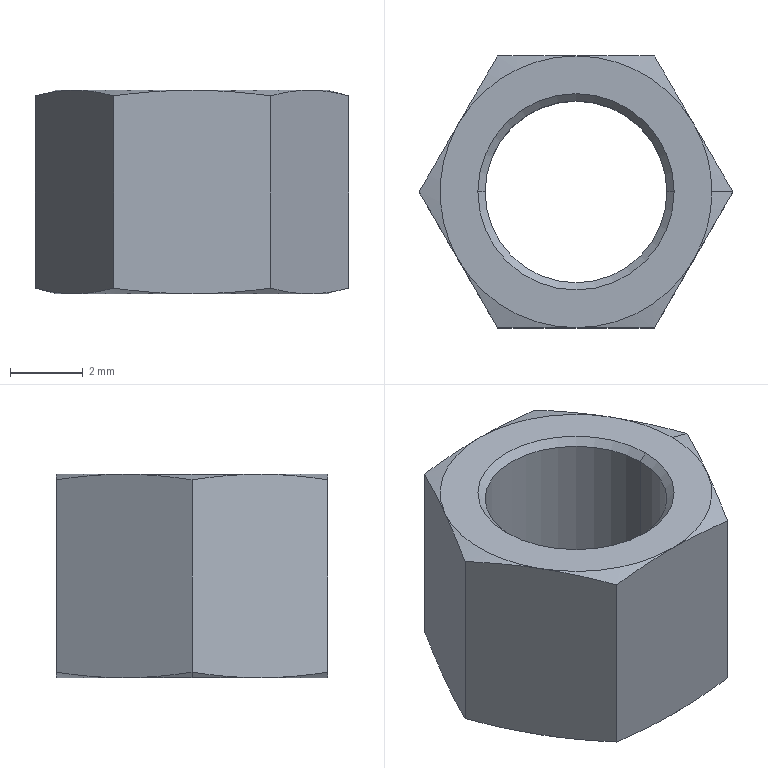Part | SolidWorks | features Cut 2, Chamfer 1, Extrusion 1 | 1 solid | 28 faces | box 8.63 x 7.474 x 5.6 mm | volume 159.862 mm3 | cone 18 | plane 8 | cylinder 2 | commonest cylinder face diameters 5 x2
STEP:
#1=CARTESIAN_POINT('',(-2.5,0.,5.4));
#2=VERTEX_POINT('',#1);
#3=CARTESIAN_POINT('',(2.5,0.,5.4));
#4=VERTEX_POINT('',#3);
#5=CARTESIAN_POINT('',(0.,0.,5.4));
#6=DIRECTION('',(0.,0.,1.));
#7=DIRECTION('',(1.,0.,0.));
#8=AXIS2_PLACEMENT_3D('',#5,#6,#7);
#9=CIRCLE('',#8,2.5);
#10=EDGE_CURVE('',#2,#4,#9,.T.);
#11=ORIENTED_EDGE('',*,*,#10,.F.);
#12=CARTESIAN_POINT('',(-2.7,0.,5.6));
#13=VERTEX_POINT('',#12);
#14=CARTESIAN_POINT('',(-2.5,0.,5.4));
#15=DIRECTION('',(-0.7071,0.,0.7071));
#16=VECTOR('',#15,1000.);
#17=LINE('',#14,#16);
#18=EDGE_CURVE('',#2,#13,#17,.T.);
#19=ORIENTED_EDGE('',*,*,#18,.T.);
#20=CARTESIAN_POINT('',(2.7,0.,5.6));
#21=VERTEX_POINT('',#20);
#22=CARTESIAN_POINT('',(0.,0.,5.6));
#23=DIRECTION('',(0.,0.,-1.));
#24=DIRECTION('',(1.,0.,0.));
#25=AXIS2_PLACEMENT_3D('',#22,#23,#24);
#26=CIRCLE('',#25,2.7);
#27=EDGE_CURVE('',#21,#13,#26,.T.);
#28=ORIENTED_EDGE('',*,*,#27,.F.);
#29=CARTESIAN_POINT('',(2.5,0.,5.4));
#30=DIRECTION('',(0.7071,0.,0.7071));
#31=VECTOR('',#30,1000.);
#32=LINE('',#29,#31);
#33=EDGE_CURVE('',#4,#21,#32,.T.);
#34=ORIENTED_EDGE('',*,*,#33,.F.);
#35=EDGE_LOOP('',(#11,#19,#28,#34));
#36=FACE_OUTER_BOUND('',#35,.T.);
#37=CARTESIAN_POINT('',(0.,0.,5.4));
#38=DIRECTION('',(0.,0.,1.));
#39=DIRECTION('',(1.,0.,0.));
#40=AXIS2_PLACEMENT_3D('',#37,#38,#39);
#41=CONICAL_SURFACE('',#40,2.5,0.7854);
#42=ADVANCED_FACE('',(#36),#41,.F.);
#43=CARTESIAN_POINT('',(2.5,0.,0.2));
#44=VERTEX_POINT('',#43);
#45=CARTESIAN_POINT('',(-2.5,0.,0.2));
#46=VERTEX_POINT('',#45);
#47=CARTESIAN_POINT('',(0.,0.,0.2));
#48=DIRECTION('',(0.,0.,-1.));
#49=DIRECTION('',(1.,0.,0.));
#50=AXIS2_PLACEMENT_3D('',#47,#48,#49);
#51=CIRCLE('',#50,2.5);
#52=EDGE_CURVE('',#44,#46,#51,.T.);
#53=ORIENTED_EDGE('',*,*,#52,.F.);
#54=CARTESIAN_POINT('',(2.7,0.,0.));
#55=VERTEX_POINT('',#54);
#56=CARTESIAN_POINT('',(2.7,0.,0.));
#57=DIRECTION('',(0.7071,0.,-0.7071));
#58=VECTOR('',#57,1000.);
#59=LINE('',#56,#58);
#60=EDGE_CURVE('',#44,#55,#59,.T.);
#61=ORIENTED_EDGE('',*,*,#60,.T.);
#62=CARTESIAN_POINT('',(-2.7,0.,0.));
#63=VERTEX_POINT('',#62);
#64=CARTESIAN_POINT('',(0.,0.,0.));
#65=DIRECTION('',(0.,0.,1.));
#66=DIRECTION('',(1.,0.,0.));
#67=AXIS2_PLACEMENT_3D('',#64,#65,#66);
#68=CIRCLE('',#67,2.7);
#69=EDGE_CURVE('',#63,#55,#68,.T.);
#70=ORIENTED_EDGE('',*,*,#69,.F.);
#71=CARTESIAN_POINT('',(-2.7,0.,0.));
#72=DIRECTION('',(-0.7071,0.,-0.7071));
#73=VECTOR('',#72,1000.);
#74=LINE('',#71,#73);
#75=EDGE_CURVE('',#46,#63,#74,.T.);
#76=ORIENTED_EDGE('',*,*,#75,.F.);
#77=EDGE_LOOP('',(#53,#61,#70,#76));
#78=FACE_OUTER_BOUND('',#77,.T.);
#79=CARTESIAN_POINT('',(0.,0.,0.));
#80=DIRECTION('',(0.,0.,-1.));
#81=DIRECTION('',(-1.,0.,0.));
#82=AXIS2_PLACEMENT_3D('',#79,#80,#81);
#83=CONICAL_SURFACE('',#82,2.7,0.7854);
#84=ADVANCED_FACE('',(#78),#83,.F.);
#85=CARTESIAN_POINT('',(3.737,0.,5.6));
#86=VERTEX_POINT('',#85);
#87=CARTESIAN_POINT('',(3.236,1.868,5.6));
#88=VERTEX_POINT('',#87);
#89=CARTESIAN_POINT('',(0.,0.,5.6));
#90=DIRECTION('',(0.,0.,1.));
#91=DIRECTION('',(1.,0.,0.));
#92=AXIS2_PLACEMENT_3D('',#89,#90,#91);
#93=CIRCLE('',#92,3.737);
#94=EDGE_CURVE('',#86,#88,#93,.T.);
#95=ORIENTED_EDGE('',*,*,#94,.F.);
#96=CARTESIAN_POINT('',(4.315,0.,5.445));
#97=VERTEX_POINT('',#96);
#98=CARTESIAN_POINT('',(3.737,0.,5.6));
#99=DIRECTION('',(0.9659,0.,-0.2588));
#100=VECTOR('',#99,1000.);
#101=LINE('',#98,#100);
#102=EDGE_CURVE('',#86,#97,#101,.T.);
#103=ORIENTED_EDGE('',*,*,#102,.T.);
#104=CARTESIAN_POINT('',(4.315,0.,5.445));
#105=CARTESIAN_POINT('',(3.955,0.6228,5.541));
#106=CARTESIAN_POINT('',(3.596,1.246,5.6));
#107=CARTESIAN_POINT('',(3.236,1.868,5.6));
#108=B_SPLINE_CURVE_WITH_KNOTS('',3,(#104,#105,#106,#107),.UNSPECIFIED.,.F.,.F.,(4,4),(0.000000231,0.002158),.UNSPECIFIED.);
#109=EDGE_CURVE('',#97,#88,#108,.T.);
#110=ORIENTED_EDGE('',*,*,#109,.T.);
#111=EDGE_LOOP('',(#95,#103,#110));
#112=FACE_OUTER_BOUND('',#111,.T.);
#113=CARTESIAN_POINT('',(0.,0.,5.6));
#114=DIRECTION('',(0.,0.,-1.));
#115=DIRECTION('',(1.,0.,0.));
#116=AXIS2_PLACEMENT_3D('',#113,#114,#115);
#117=CONICAL_SURFACE('',#116,3.737,1.309);
#118=ADVANCED_FACE('',(#112),#117,.T.);
#119=CARTESIAN_POINT('',(-3.737,0.,0.));
#120=VERTEX_POINT('',#119);
#121=CARTESIAN_POINT('',(-3.236,1.868,0.));
#122=VERTEX_POINT('',#121);
#123=CARTESIAN_POINT('',(0.,0.,0.));
#124=DIRECTION('',(0.,0.,-1.));
#125=DIRECTION('',(-1.,0.,0.));
#126=AXIS2_PLACEMENT_3D('',#123,#124,#125);
#127=CIRCLE('',#126,3.737);
#128=EDGE_CURVE('',#120,#122,#127,.T.);
#129=ORIENTED_EDGE('',*,*,#128,.F.);
#130=CARTESIAN_POINT('',(-4.315,0.,0.1549));
#131=VERTEX_POINT('',#130);
#132=CARTESIAN_POINT('',(-3.737,0.,0.));
#133=DIRECTION('',(-0.9659,0.,0.2588));
#134=VECTOR('',#133,1000.);
#135=LINE('',#132,#134);
#136=EDGE_CURVE('',#120,#131,#135,.T.);
#137=ORIENTED_EDGE('',*,*,#136,.T.);
#138=CARTESIAN_POINT('',(-4.315,0.,0.1549));
#139=CARTESIAN_POINT('',(-3.955,0.6228,0.05855));
#140=CARTESIAN_POINT('',(-3.596,1.246,0.));
#141=CARTESIAN_POINT('',(-3.236,1.868,0.));
#142=B_SPLINE_CURVE_WITH_KNOTS('',3,(#138,#139,#140,#141),.UNSPECIFIED.,.F.,.F.,(4,4),(0.000000231,0.002158),.UNSPECIFIED.);
#143=EDGE_CURVE('',#131,#122,#142,.T.);
#144=ORIENTED_EDGE('',*,*,#143,.T.);
#145=EDGE_LOOP('',(#129,#137,#144));
#146=FACE_OUTER_BOUND('',#145,.T.);
#147=CARTESIAN_POINT('',(0.,0.,0.));
#148=DIRECTION('',(0.,0.,1.));
#149=DIRECTION('',(-1.,0.,0.));
#150=AXIS2_PLACEMENT_3D('',#147,#148,#149);
#151=CONICAL_SURFACE('',#150,3.737,1.309);
#152=ADVANCED_FACE('',(#146),#151,.T.);
#153=ORIENTED_EDGE('',*,*,#10,.T.);
#154=CARTESIAN_POINT('',(2.5,0.,5.6));
#155=DIRECTION('',(0.,0.,-1.));
#156=VECTOR('',#155,1000.);
#157=LINE('',#154,#156);
#158=EDGE_CURVE('',#4,#44,#157,.T.);
#159=ORIENTED_EDGE('',*,*,#158,.T.);
#160=ORIENTED_EDGE('',*,*,#52,.T.);
#161=CARTESIAN_POINT('',(-2.5,0.,5.6));
#162=DIRECTION('',(0.,0.,-1.));
#163=VECTOR('',#162,1000.);
#164=LINE('',#161,#163);
#165=EDGE_CURVE('',#2,#46,#164,.T.);
#166=ORIENTED_EDGE('',*,*,#165,.F.);
#167=EDGE_LOOP('',(#153,#159,#160,#166));
#168=FACE_OUTER_BOUND('',#167,.T.);
#169=CARTESIAN_POINT('',(0.,0.,5.6));
#170=DIRECTION('',(0.,0.,-1.));
#171=DIRECTION('',(-1.,0.,0.));
#172=AXIS2_PLACEMENT_3D('',#169,#170,#171);
#173=CYLINDRICAL_SURFACE('',#172,2.5);
#174=ADVANCED_FACE('',(#168),#173,.F.);
#175=ORIENTED_EDGE('',*,*,#109,.F.);
#176=CARTESIAN_POINT('',(4.315,0.,0.1549));
#177=VERTEX_POINT('',#176);
#178=CARTESIAN_POINT('',(4.315,0.,5.6));
#179=DIRECTION('',(0.,0.,-1.));
#180=VECTOR('',#179,1000.);
#181=LINE('',#178,#180);
#182=EDGE_CURVE('',#97,#177,#181,.T.);
#183=ORIENTED_EDGE('',*,*,#182,.T.);
#184=CARTESIAN_POINT('',(3.236,1.868,0.));
#185=VERTEX_POINT('',#184);
#186=CARTESIAN_POINT('',(3.236,1.868,0.));
#187=CARTESIAN_POINT('',(3.596,1.246,0.));
#188=CARTESIAN_POINT('',(3.955,0.6228,0.05855));
#189=CARTESIAN_POINT('',(4.315,0.,0.1549));
#190=B_SPLINE_CURVE_WITH_KNOTS('',3,(#186,#187,#188,#189),.UNSPECIFIED.,.F.,.F.,(4,4),(0.002158,0.004315),.UNSPECIFIED.);
#191=EDGE_CURVE('',#185,#177,#190,.T.);
#192=ORIENTED_EDGE('',*,*,#191,.F.);
#193=CARTESIAN_POINT('',(2.158,3.737,0.1549));
#194=VERTEX_POINT('',#193);
#195=CARTESIAN_POINT('',(2.158,3.737,0.1549));
#196=CARTESIAN_POINT('',(2.517,3.114,0.05855));
#197=CARTESIAN_POINT('',(2.877,2.491,0.));
#198=CARTESIAN_POINT('',(3.236,1.868,0.));
#199=B_SPLINE_CURVE_WITH_KNOTS('',3,(#195,#196,#197,#198),.UNSPECIFIED.,.F.,.F.,(4,4),(0.000000231,0.002158),.UNSPECIFIED.);
#200=EDGE_CURVE('',#194,#185,#199,.T.);
#201=ORIENTED_EDGE('',*,*,#200,.F.);
#202=CARTESIAN_POINT('',(2.158,3.737,5.445));
#203=VERTEX_POINT('',#202);
#204=CARTESIAN_POINT('',(2.158,3.737,5.6));
#205=DIRECTION('',(0.,0.,-1.));
#206=VECTOR('',#205,1000.);
#207=LINE('',#204,#206);
#208=EDGE_CURVE('',#203,#194,#207,.T.);
#209=ORIENTED_EDGE('',*,*,#208,.F.);
#210=CARTESIAN_POINT('',(3.236,1.868,5.6));
#211=CARTESIAN_POINT('',(2.877,2.491,5.6));
#212=CARTESIAN_POINT('',(2.517,3.114,5.541));
#213=CARTESIAN_POINT('',(2.158,3.737,5.445));
#214=B_SPLINE_CURVE_WITH_KNOTS('',3,(#210,#211,#212,#213),.UNSPECIFIED.,.F.,.F.,(4,4),(0.002158,0.004315),.UNSPECIFIED.);
#215=EDGE_CURVE('',#88,#203,#214,.T.);
#216=ORIENTED_EDGE('',*,*,#215,.F.);
#217=EDGE_LOOP('',(#175,#183,#192,#201,#209,#216));
#218=FACE_OUTER_BOUND('',#217,.T.);
#219=CARTESIAN_POINT('',(4.315,0.,5.6));
#220=DIRECTION('',(-0.866,-0.5,0.));
#221=DIRECTION('',(0.5,-0.866,0.));
#222=AXIS2_PLACEMENT_3D('',#219,#220,#221);
#223=PLANE('',#222);
#224=ADVANCED_FACE('',(#218),#223,.F.);
#225=CARTESIAN_POINT('',(0.,3.737,5.6));
#226=VERTEX_POINT('',#225);
#227=CARTESIAN_POINT('',(2.158,3.737,5.445));
#228=CARTESIAN_POINT('',(1.44,3.737,5.541));
#229=CARTESIAN_POINT('',(0.7205,3.737,5.6));
#230=CARTESIAN_POINT('',(0.,3.737,5.6));
#231=B_SPLINE_CURVE_WITH_KNOTS('',3,(#227,#228,#229,#230),.UNSPECIFIED.,.F.,.F.,(4,4),(0.01379,0.01596),.UNSPECIFIED.);
#232=EDGE_CURVE('',#203,#226,#231,.T.);
#233=ORIENTED_EDGE('',*,*,#232,.F.);
#234=ORIENTED_EDGE('',*,*,#208,.T.);
#235=CARTESIAN_POINT('',(0.,3.737,0.));
#236=VERTEX_POINT('',#235);
#237=CARTESIAN_POINT('',(0.,3.737,0.));
#238=CARTESIAN_POINT('',(0.7205,3.737,0.));
#239=CARTESIAN_POINT('',(1.44,3.737,0.05871));
#240=CARTESIAN_POINT('',(2.158,3.737,0.1549));
#241=B_SPLINE_CURVE_WITH_KNOTS('',3,(#237,#238,#239,#240),.UNSPECIFIED.,.F.,.F.,(4,4),(0.00587,0.008046),.UNSPECIFIED.);
#242=EDGE_CURVE('',#236,#194,#241,.T.);
#243=ORIENTED_EDGE('',*,*,#242,.F.);
#244=CARTESIAN_POINT('',(-2.157,3.737,0.1549));
#245=VERTEX_POINT('',#244);
#246=CARTESIAN_POINT('',(-2.157,3.737,0.1549));
#247=CARTESIAN_POINT('',(-1.44,3.737,0.05881));
#248=CARTESIAN_POINT('',(-0.7182,3.737,0.));
#249=CARTESIAN_POINT('',(0.,3.737,0.));
#250=B_SPLINE_CURVE_WITH_KNOTS('',3,(#246,#247,#248,#249),.UNSPECIFIED.,.F.,.F.,(4,4),(0.003702,0.00587),.UNSPECIFIED.);
#251=EDGE_CURVE('',#245,#236,#250,.T.);
#252=ORIENTED_EDGE('',*,*,#251,.F.);
#253=CARTESIAN_POINT('',(-2.157,3.737,5.445));
#254=VERTEX_POINT('',#253);
#255=CARTESIAN_POINT('',(-2.157,3.737,5.6));
#256=DIRECTION('',(0.,0.,-1.));
#257=VECTOR('',#256,1000.);
#258=LINE('',#255,#257);
#259=EDGE_CURVE('',#254,#245,#258,.T.);
#260=ORIENTED_EDGE('',*,*,#259,.F.);
#261=CARTESIAN_POINT('',(0.,3.737,5.6));
#262=CARTESIAN_POINT('',(-0.7182,3.737,5.6));
#263=CARTESIAN_POINT('',(-1.44,3.737,5.541));
#264=CARTESIAN_POINT('',(-2.157,3.737,5.445));
#265=B_SPLINE_CURVE_WITH_KNOTS('',3,(#261,#262,#263,#264),.UNSPECIFIED.,.F.,.F.,(4,4),(0.01596,0.01813),.UNSPECIFIED.);
#266=EDGE_CURVE('',#226,#254,#265,.T.);
#267=ORIENTED_EDGE('',*,*,#266,.F.);
#268=EDGE_LOOP('',(#233,#234,#243,#252,#260,#267));
#269=FACE_OUTER_BOUND('',#268,.T.);
#270=CARTESIAN_POINT('',(2.158,3.737,5.6));
#271=DIRECTION('',(0.,-1.,0.));
#272=DIRECTION('',(0.,0.,-1.));
#273=AXIS2_PLACEMENT_3D('',#270,#271,#272);
#274=PLANE('',#273);
#275=ADVANCED_FACE('',(#269),#274,.F.);
#276=CARTESIAN_POINT('',(-3.236,1.868,5.6));
#277=VERTEX_POINT('',#276);
#278=CARTESIAN_POINT('',(-2.157,3.737,5.445));
#279=CARTESIAN_POINT('',(-2.517,3.114,5.541));
#280=CARTESIAN_POINT('',(-2.877,2.491,5.6));
#281=CARTESIAN_POINT('',(-3.236,1.868,5.6));
#282=B_SPLINE_CURVE_WITH_KNOTS('',3,(#278,#279,#280,#281),.UNSPECIFIED.,.F.,.F.,(4,4),(0.000000231,0.002158),.UNSPECIFIED.);
#283=EDGE_CURVE('',#254,#277,#282,.T.);
#284=ORIENTED_EDGE('',*,*,#283,.F.);
#285=ORIENTED_EDGE('',*,*,#259,.T.);
#286=CARTESIAN_POINT('',(-3.236,1.868,0.));
#287=CARTESIAN_POINT('',(-2.877,2.491,0.));
#288=CARTESIAN_POINT('',(-2.517,3.114,0.05855));
#289=CARTESIAN_POINT('',(-2.157,3.737,0.1549));
#290=B_SPLINE_CURVE_WITH_KNOTS('',3,(#286,#287,#288,#289),.UNSPECIFIED.,.F.,.F.,(4,4),(0.002158,0.004315),.UNSPECIFIED.);
#291=EDGE_CURVE('',#122,#245,#290,.T.);
#292=ORIENTED_EDGE('',*,*,#291,.F.);
#293=ORIENTED_EDGE('',*,*,#143,.F.);
#294=CARTESIAN_POINT('',(-4.315,0.,5.445));
#295=VERTEX_POINT('',#294);
#296=CARTESIAN_POINT('',(-4.315,0.,5.6));
#297=DIRECTION('',(0.,0.,-1.));
#298=VECTOR('',#297,1000.);
#299=LINE('',#296,#298);
#300=EDGE_CURVE('',#295,#131,#299,.T.);
#301=ORIENTED_EDGE('',*,*,#300,.F.);
#302=CARTESIAN_POINT('',(-3.236,1.868,5.6));
#303=CARTESIAN_POINT('',(-3.596,1.246,5.6));
#304=CARTESIAN_POINT('',(-3.955,0.6228,5.541));
#305=CARTESIAN_POINT('',(-4.315,0.,5.445));
#306=B_SPLINE_CURVE_WITH_KNOTS('',3,(#302,#303,#304,#305),.UNSPECIFIED.,.F.,.F.,(4,4),(0.002158,0.004315),.UNSPECIFIED.);
#307=EDGE_CURVE('',#277,#295,#306,.T.);
#308=ORIENTED_EDGE('',*,*,#307,.F.);
#309=EDGE_LOOP('',(#284,#285,#292,#293,#301,#308));
#310=FACE_OUTER_BOUND('',#309,.T.);
#311=CARTESIAN_POINT('',(-2.157,3.737,5.6));
#312=DIRECTION('',(0.866,-0.5,0.));
#313=DIRECTION('',(0.5,0.866,0.));
#314=AXIS2_PLACEMENT_3D('',#311,#312,#313);
#315=PLANE('',#314);
#316=ADVANCED_FACE('',(#310),#315,.F.);
#317=CARTESIAN_POINT('',(-3.236,-1.868,5.6));
#318=VERTEX_POINT('',#317);
#319=CARTESIAN_POINT('',(-4.315,0.,5.445));
#320=CARTESIAN_POINT('',(-3.955,-0.6228,5.541));
#321=CARTESIAN_POINT('',(-3.596,-1.246,5.6));
#322=CARTESIAN_POINT('',(-3.236,-1.868,5.6));
#323=B_SPLINE_CURVE_WITH_KNOTS('',3,(#319,#320,#321,#322),.UNSPECIFIED.,.F.,.F.,(4,4),(0.000000231,0.002158),.UNSPECIFIED.);
#324=EDGE_CURVE('',#295,#318,#323,.T.);
#325=ORIENTED_EDGE('',*,*,#324,.F.);
#326=ORIENTED_EDGE('',*,*,#300,.T.);
#327=CARTESIAN_POINT('',(-3.236,-1.868,0.));
#328=VERTEX_POINT('',#327);
#329=CARTESIAN_POINT('',(-3.236,-1.868,0.));
#330=CARTESIAN_POINT('',(-3.596,-1.246,0.));
#331=CARTESIAN_POINT('',(-3.955,-0.6228,0.05855));
#332=CARTESIAN_POINT('',(-4.315,0.,0.1549));
#333=B_SPLINE_CURVE_WITH_KNOTS('',3,(#329,#330,#331,#332),.UNSPECIFIED.,.F.,.F.,(4,4),(0.002158,0.004315),.UNSPECIFIED.);
#334=EDGE_CURVE('',#328,#131,#333,.T.);
#335=ORIENTED_EDGE('',*,*,#334,.F.);
#336=CARTESIAN_POINT('',(-2.157,-3.737,0.1549));
#337=VERTEX_POINT('',#336);
#338=CARTESIAN_POINT('',(-2.157,-3.737,0.1549));
#339=CARTESIAN_POINT('',(-2.517,-3.114,0.05855));
#340=CARTESIAN_POINT('',(-2.877,-2.491,0.));
#341=CARTESIAN_POINT('',(-3.236,-1.868,0.));
#342=B_SPLINE_CURVE_WITH_KNOTS('',3,(#338,#339,#340,#341),.UNSPECIFIED.,.F.,.F.,(4,4),(0.000000231,0.002158),.UNSPECIFIED.);
#343=EDGE_CURVE('',#337,#328,#342,.T.);
#344=ORIENTED_EDGE('',*,*,#343,.F.);
#345=CARTESIAN_POINT('',(-2.157,-3.737,5.445));
#346=VERTEX_POINT('',#345);
#347=CARTESIAN_POINT('',(-2.157,-3.737,5.6));
#348=DIRECTION('',(0.,0.,-1.));
#349=VECTOR('',#348,1000.);
#350=LINE('',#347,#349);
#351=EDGE_CURVE('',#346,#337,#350,.T.);
#352=ORIENTED_EDGE('',*,*,#351,.F.);
#353=CARTESIAN_POINT('',(-3.236,-1.868,5.6));
#354=CARTESIAN_POINT('',(-2.877,-2.491,5.6));
#355=CARTESIAN_POINT('',(-2.517,-3.114,5.541));
#356=CARTESIAN_POINT('',(-2.157,-3.737,5.445));
#357=B_SPLINE_CURVE_WITH_KNOTS('',3,(#353,#354,#355,#356),.UNSPECIFIED.,.F.,.F.,(4,4),(0.002158,0.004315),.UNSPECIFIED.);
#358=EDGE_CURVE('',#318,#346,#357,.T.);
#359=ORIENTED_EDGE('',*,*,#358,.F.);
#360=EDGE_LOOP('',(#325,#326,#335,#344,#352,#359));
#361=FACE_OUTER_BOUND('',#360,.T.);
#362=CARTESIAN_POINT('',(-4.315,0.,5.6));
#363=DIRECTION('',(0.866,0.5,0.));
#364=DIRECTION('',(-0.5,0.866,0.));
#365=AXIS2_PLACEMENT_3D('',#362,#363,#364);
#366=PLANE('',#365);
#367=ADVANCED_FACE('',(#361),#366,.F.);
#368=CARTESIAN_POINT('',(0.,-3.737,5.6));
#369=VERTEX_POINT('',#368);
#370=CARTESIAN_POINT('',(-2.157,-3.737,5.445));
#371=CARTESIAN_POINT('',(-1.44,-3.737,5.541));
#372=CARTESIAN_POINT('',(-0.7182,-3.737,5.6));
#373=CARTESIAN_POINT('',(0.,-3.737,5.6));
#374=B_SPLINE_CURVE_WITH_KNOTS('',3,(#370,#371,#372,#373),.UNSPECIFIED.,.F.,.F.,(4,4),(0.003702,0.00587),.UNSPECIFIED.);
#375=EDGE_CURVE('',#346,#369,#374,.T.);
#376=ORIENTED_EDGE('',*,*,#375,.F.);
#377=ORIENTED_EDGE('',*,*,#351,.T.);
#378=CARTESIAN_POINT('',(0.,-3.737,0.));
#379=VERTEX_POINT('',#378);
#380=CARTESIAN_POINT('',(0.,-3.737,0.));
#381=CARTESIAN_POINT('',(-0.7182,-3.737,0.));
#382=CARTESIAN_POINT('',(-1.44,-3.737,0.05881));
#383=CARTESIAN_POINT('',(-2.157,-3.737,0.1549));
#384=B_SPLINE_CURVE_WITH_KNOTS('',3,(#380,#381,#382,#383),.UNSPECIFIED.,.F.,.F.,(4,4),(0.01596,0.01813),.UNSPECIFIED.);
#385=EDGE_CURVE('',#379,#337,#384,.T.);
#386=ORIENTED_EDGE('',*,*,#385,.F.);
#387=CARTESIAN_POINT('',(2.158,-3.737,0.1549));
#388=VERTEX_POINT('',#387);
#389=CARTESIAN_POINT('',(2.158,-3.737,0.1549));
#390=CARTESIAN_POINT('',(1.44,-3.737,0.05871));
#391=CARTESIAN_POINT('',(0.7205,-3.737,0.));
#392=CARTESIAN_POINT('',(0.,-3.737,0.));
#393=B_SPLINE_CURVE_WITH_KNOTS('',3,(#389,#390,#391,#392),.UNSPECIFIED.,.F.,.F.,(4,4),(0.01379,0.01596),.UNSPECIFIED.);
#394=EDGE_CURVE('',#388,#379,#393,.T.);
#395=ORIENTED_EDGE('',*,*,#394,.F.);
#396=CARTESIAN_POINT('',(2.158,-3.737,5.445));
#397=VERTEX_POINT('',#396);
#398=CARTESIAN_POINT('',(2.158,-3.737,5.6));
#399=DIRECTION('',(0.,0.,-1.));
#400=VECTOR('',#399,1000.);
#401=LINE('',#398,#400);
#402=EDGE_CURVE('',#397,#388,#401,.T.);
#403=ORIENTED_EDGE('',*,*,#402,.F.);
#404=CARTESIAN_POINT('',(0.,-3.737,5.6));
#405=CARTESIAN_POINT('',(0.7205,-3.737,5.6));
#406=CARTESIAN_POINT('',(1.44,-3.737,5.541));
#407=CARTESIAN_POINT('',(2.158,-3.737,5.445));
#408=B_SPLINE_CURVE_WITH_KNOTS('',3,(#404,#405,#406,#407),.UNSPECIFIED.,.F.,.F.,(4,4),(0.00587,0.008046),.UNSPECIFIED.);
#409=EDGE_CURVE('',#369,#397,#408,.T.);
#410=ORIENTED_EDGE('',*,*,#409,.F.);
#411=EDGE_LOOP('',(#376,#377,#386,#395,#403,#410));
#412=FACE_OUTER_BOUND('',#411,.T.);
#413=CARTESIAN_POINT('',(-2.157,-3.737,5.6));
#414=DIRECTION('',(0.,1.,0.));
#415=DIRECTION('',(0.,0.,1.));
#416=AXIS2_PLACEMENT_3D('',#413,#414,#415);
#417=PLANE('',#416);
#418=ADVANCED_FACE('',(#412),#417,.F.);
#419=CARTESIAN_POINT('',(3.236,-1.868,5.6));
#420=VERTEX_POINT('',#419);
#421=CARTESIAN_POINT('',(2.158,-3.737,5.445));
#422=CARTESIAN_POINT('',(2.517,-3.114,5.541));
#423=CARTESIAN_POINT('',(2.877,-2.491,5.6));
#424=CARTESIAN_POINT('',(3.236,-1.868,5.6));
#425=B_SPLINE_CURVE_WITH_KNOTS('',3,(#421,#422,#423,#424),.UNSPECIFIED.,.F.,.F.,(4,4),(0.000000231,0.002158),.UNSPECIFIED.);
#426=EDGE_CURVE('',#397,#420,#425,.T.);
#427=ORIENTED_EDGE('',*,*,#426,.F.);
#428=ORIENTED_EDGE('',*,*,#402,.T.);
#429=CARTESIAN_POINT('',(3.236,-1.868,0.));
#430=VERTEX_POINT('',#429);
#431=CARTESIAN_POINT('',(3.236,-1.868,0.));
#432=CARTESIAN_POINT('',(2.877,-2.491,0.));
#433=CARTESIAN_POINT('',(2.517,-3.114,0.05855));
#434=CARTESIAN_POINT('',(2.158,-3.737,0.1549));
#435=B_SPLINE_CURVE_WITH_KNOTS('',3,(#431,#432,#433,#434),.UNSPECIFIED.,.F.,.F.,(4,4),(0.002158,0.004315),.UNSPECIFIED.);
#436=EDGE_CURVE('',#430,#388,#435,.T.);
#437=ORIENTED_EDGE('',*,*,#436,.F.);
#438=CARTESIAN_POINT('',(4.315,0.,0.1549));
#439=CARTESIAN_POINT('',(3.955,-0.6228,0.05855));
#440=CARTESIAN_POINT('',(3.596,-1.246,0.));
#441=CARTESIAN_POINT('',(3.236,-1.868,0.));
#442=B_SPLINE_CURVE_WITH_KNOTS('',3,(#438,#439,#440,#441),.UNSPECIFIED.,.F.,.F.,(4,4),(0.000000231,0.002158),.UNSPECIFIED.);
#443=EDGE_CURVE('',#177,#430,#442,.T.);
#444=ORIENTED_EDGE('',*,*,#443,.F.);
#445=ORIENTED_EDGE('',*,*,#182,.F.);
#446=CARTESIAN_POINT('',(3.236,-1.868,5.6));
#447=CARTESIAN_POINT('',(3.596,-1.246,5.6));
#448=CARTESIAN_POINT('',(3.955,-0.6228,5.541));
#449=CARTESIAN_POINT('',(4.315,0.,5.445));
#450=B_SPLINE_CURVE_WITH_KNOTS('',3,(#446,#447,#448,#449),.UNSPECIFIED.,.F.,.F.,(4,4),(0.002158,0.004315),.UNSPECIFIED.);
#451=EDGE_CURVE('',#420,#97,#450,.T.);
#452=ORIENTED_EDGE('',*,*,#451,.F.);
#453=EDGE_LOOP('',(#427,#428,#437,#444,#445,#452));
#454=FACE_OUTER_BOUND('',#453,.T.);
#455=CARTESIAN_POINT('',(2.158,-3.737,5.6));
#456=DIRECTION('',(-0.866,0.5,0.));
#457=DIRECTION('',(-0.5,-0.866,0.));
#458=AXIS2_PLACEMENT_3D('',#455,#456,#457);
#459=PLANE('',#458);
#460=ADVANCED_FACE('',(#454),#459,.F.);
#461=ORIENTED_EDGE('',*,*,#27,.T.);
#462=CARTESIAN_POINT('',(0.,0.,5.6));
#463=DIRECTION('',(0.,0.,-1.));
#464=DIRECTION('',(1.,0.,0.));
#465=AXIS2_PLACEMENT_3D('',#462,#463,#464);
#466=CIRCLE('',#465,2.7);
#467=EDGE_CURVE('',#13,#21,#466,.T.);
#468=ORIENTED_EDGE('',*,*,#467,.T.);
#469=EDGE_LOOP('',(#461,#468));
#470=FACE_BOUND('',#469,.T.);
#471=CARTESIAN_POINT('',(0.,0.,5.6));
#472=DIRECTION('',(0.,0.,1.));
#473=DIRECTION('',(1.,0.,0.));
#474=AXIS2_PLACEMENT_3D('',#471,#472,#473);
#475=CIRCLE('',#474,3.737);
#476=EDGE_CURVE('',#420,#86,#475,.T.);
#477=ORIENTED_EDGE('',*,*,#476,.T.);
#478=ORIENTED_EDGE('',*,*,#94,.T.);
#479=CARTESIAN_POINT('',(0.,0.,5.6));
#480=DIRECTION('',(0.,0.,1.));
#481=DIRECTION('',(1.,0.,0.));
#482=AXIS2_PLACEMENT_3D('',#479,#480,#481);
#483=CIRCLE('',#482,3.737);
#484=EDGE_CURVE('',#88,#226,#483,.T.);
#485=ORIENTED_EDGE('',*,*,#484,.T.);
#486=CARTESIAN_POINT('',(0.,0.,5.6));
#487=DIRECTION('',(0.,0.,1.));
#488=DIRECTION('',(1.,0.,0.));
#489=AXIS2_PLACEMENT_3D('',#486,#487,#488);
#490=CIRCLE('',#489,3.737);
#491=EDGE_CURVE('',#226,#277,#490,.T.);
#492=ORIENTED_EDGE('',*,*,#491,.T.);
#493=CARTESIAN_POINT('',(0.,0.,5.6));
#494=DIRECTION('',(0.,0.,1.));
#495=DIRECTION('',(1.,0.,0.));
#496=AXIS2_PLACEMENT_3D('',#493,#494,#495);
#497=CIRCLE('',#496,3.737);
#498=EDGE_CURVE('',#277,#318,#497,.T.);
#499=ORIENTED_EDGE('',*,*,#498,.T.);
#500=CARTESIAN_POINT('',(0.,0.,5.6));
#501=DIRECTION('',(0.,0.,1.));
#502=DIRECTION('',(1.,0.,0.));
#503=AXIS2_PLACEMENT_3D('',#500,#501,#502);
#504=CIRCLE('',#503,3.737);
#505=EDGE_CURVE('',#318,#369,#504,.T.);
#506=ORIENTED_EDGE('',*,*,#505,.T.);
#507=CARTESIAN_POINT('',(0.,0.,5.6));
#508=DIRECTION('',(0.,0.,1.));
#509=DIRECTION('',(1.,0.,0.));
#510=AXIS2_PLACEMENT_3D('',#507,#508,#509);
#511=CIRCLE('',#510,3.737);
#512=EDGE_CURVE('',#369,#420,#511,.T.);
#513=ORIENTED_EDGE('',*,*,#512,.T.);
#514=EDGE_LOOP('',(#477,#478,#485,#492,#499,#506,#513));
#515=FACE_OUTER_BOUND('',#514,.T.);
#516=CARTESIAN_POINT('',(2.158,3.737,5.6));
#517=DIRECTION('',(0.,0.,1.));
#518=DIRECTION('',(1.,0.,0.));
#519=AXIS2_PLACEMENT_3D('',#516,#517,#518);
#520=PLANE('',#519);
#521=ADVANCED_FACE('',(#470,#515),#520,.T.);
#522=ORIENTED_EDGE('',*,*,#69,.T.);
#523=CARTESIAN_POINT('',(0.,0.,0.));
#524=DIRECTION('',(0.,0.,1.));
#525=DIRECTION('',(1.,0.,0.));
#526=AXIS2_PLACEMENT_3D('',#523,#524,#525);
#527=CIRCLE('',#526,2.7);
#528=EDGE_CURVE('',#55,#63,#527,.T.);
#529=ORIENTED_EDGE('',*,*,#528,.T.);
#530=EDGE_LOOP('',(#522,#529));
#531=FACE_BOUND('',#530,.T.);
#532=CARTESIAN_POINT('',(0.,0.,0.));
#533=DIRECTION('',(0.,0.,-1.));
#534=DIRECTION('',(-1.,0.,0.));
#535=AXIS2_PLACEMENT_3D('',#532,#533,#534);
#536=CIRCLE('',#535,3.737);
#537=EDGE_CURVE('',#236,#185,#536,.T.);
#538=ORIENTED_EDGE('',*,*,#537,.T.);
#539=CARTESIAN_POINT('',(0.,0.,0.));
#540=DIRECTION('',(0.,0.,-1.));
#541=DIRECTION('',(-1.,0.,0.));
#542=AXIS2_PLACEMENT_3D('',#539,#540,#541);
#543=CIRCLE('',#542,3.737);
#544=EDGE_CURVE('',#185,#430,#543,.T.);
#545=ORIENTED_EDGE('',*,*,#544,.T.);
#546=CARTESIAN_POINT('',(0.,0.,0.));
#547=DIRECTION('',(0.,0.,-1.));
#548=DIRECTION('',(-1.,0.,0.));
#549=AXIS2_PLACEMENT_3D('',#546,#547,#548);
#550=CIRCLE('',#549,3.737);
#551=EDGE_CURVE('',#430,#379,#550,.T.);
#552=ORIENTED_EDGE('',*,*,#551,.T.);
#553=CARTESIAN_POINT('',(0.,0.,0.));
#554=DIRECTION('',(0.,0.,-1.));
#555=DIRECTION('',(-1.,0.,0.));
#556=AXIS2_PLACEMENT_3D('',#553,#554,#555);
#557=CIRCLE('',#556,3.737);
#558=EDGE_CURVE('',#379,#328,#557,.T.);
#559=ORIENTED_EDGE('',*,*,#558,.T.);
#560=CARTESIAN_POINT('',(0.,0.,0.));
#561=DIRECTION('',(0.,0.,-1.));
#562=DIRECTION('',(-1.,0.,0.));
#563=AXIS2_PLACEMENT_3D('',#560,#561,#562);
#564=CIRCLE('',#563,3.737);
#565=EDGE_CURVE('',#328,#120,#564,.T.);
#566=ORIENTED_EDGE('',*,*,#565,.T.);
#567=ORIENTED_EDGE('',*,*,#128,.T.);
#568=CARTESIAN_POINT('',(0.,0.,0.));
#569=DIRECTION('',(0.,0.,-1.));
#570=DIRECTION('',(-1.,0.,0.));
#571=AXIS2_PLACEMENT_3D('',#568,#569,#570);
#572=CIRCLE('',#571,3.737);
#573=EDGE_CURVE('',#122,#236,#572,.T.);
#574=ORIENTED_EDGE('',*,*,#573,.T.);
#575=EDGE_LOOP('',(#538,#545,#552,#559,#566,#567,#574));
#576=FACE_OUTER_BOUND('',#575,.T.);
#577=CARTESIAN_POINT('',(2.158,3.737,0.));
#578=DIRECTION('',(0.,0.,1.));
#579=DIRECTION('',(1.,0.,0.));
#580=AXIS2_PLACEMENT_3D('',#577,#578,#579);
#581=PLANE('',#580);
#582=ADVANCED_FACE('',(#531,#576),#581,.F.);
#583=ORIENTED_EDGE('',*,*,#158,.F.);
#584=CARTESIAN_POINT('',(0.,0.,5.4));
#585=DIRECTION('',(0.,0.,1.));
#586=DIRECTION('',(1.,0.,0.));
#587=AXIS2_PLACEMENT_3D('',#584,#585,#586);
#588=CIRCLE('',#587,2.5);
#589=EDGE_CURVE('',#4,#2,#588,.T.);
#590=ORIENTED_EDGE('',*,*,#589,.T.);
#591=ORIENTED_EDGE('',*,*,#165,.T.);
#592=CARTESIAN_POINT('',(0.,0.,0.2));
#593=DIRECTION('',(0.,0.,-1.));
#594=DIRECTION('',(1.,0.,0.));
#595=AXIS2_PLACEMENT_3D('',#592,#593,#594);
#596=CIRCLE('',#595,2.5);
#597=EDGE_CURVE('',#46,#44,#596,.T.);
#598=ORIENTED_EDGE('',*,*,#597,.T.);
#599=EDGE_LOOP('',(#583,#590,#591,#598));
#600=FACE_OUTER_BOUND('',#599,.T.);
#601=CARTESIAN_POINT('',(0.,0.,5.6));
#602=DIRECTION('',(0.,0.,-1.));
#603=DIRECTION('',(-1.,0.,0.));
#604=AXIS2_PLACEMENT_3D('',#601,#602,#603);
#605=CYLINDRICAL_SURFACE('',#604,2.5);
#606=ADVANCED_FACE('',(#600),#605,.F.);
#607=ORIENTED_EDGE('',*,*,#394,.T.);
#608=ORIENTED_EDGE('',*,*,#551,.F.);
#609=ORIENTED_EDGE('',*,*,#436,.T.);
#610=EDGE_LOOP('',(#607,#608,#609));
#611=FACE_OUTER_BOUND('',#610,.T.);
#612=CARTESIAN_POINT('',(0.,0.,0.));
#613=DIRECTION('',(0.,0.,1.));
#614=DIRECTION('',(-1.,0.,0.));
#615=AXIS2_PLACEMENT_3D('',#612,#613,#614);
#616=CONICAL_SURFACE('',#615,3.737,1.309);
#617=ADVANCED_FACE('',(#611),#616,.T.);
#618=ORIENTED_EDGE('',*,*,#191,.T.);
#619=ORIENTED_EDGE('',*,*,#443,.T.);
#620=ORIENTED_EDGE('',*,*,#544,.F.);
#621=EDGE_LOOP('',(#618,#619,#620));
#622=FACE_OUTER_BOUND('',#621,.T.);
#623=CARTESIAN_POINT('',(0.,0.,0.));
#624=DIRECTION('',(0.,0.,1.));
#625=DIRECTION('',(-1.,0.,0.));
#626=AXIS2_PLACEMENT_3D('',#623,#624,#625);
#627=CONICAL_SURFACE('',#626,3.737,1.309);
#628=ADVANCED_FACE('',(#622),#627,.T.);
#629=ORIENTED_EDGE('',*,*,#343,.T.);
#630=ORIENTED_EDGE('',*,*,#558,.F.);
#631=ORIENTED_EDGE('',*,*,#385,.T.);
#632=EDGE_LOOP('',(#629,#630,#631));
#633=FACE_OUTER_BOUND('',#632,.T.);
#634=CARTESIAN_POINT('',(0.,0.,0.));
#635=DIRECTION('',(0.,0.,1.));
#636=DIRECTION('',(-1.,0.,0.));
#637=AXIS2_PLACEMENT_3D('',#634,#635,#636);
#638=CONICAL_SURFACE('',#637,3.737,1.309);
#639=ADVANCED_FACE('',(#633),#638,.T.);
#640=ORIENTED_EDGE('',*,*,#136,.F.);
#641=ORIENTED_EDGE('',*,*,#565,.F.);
#642=ORIENTED_EDGE('',*,*,#334,.T.);
#643=EDGE_LOOP('',(#640,#641,#642));
#644=FACE_OUTER_BOUND('',#643,.T.);
#645=CARTESIAN_POINT('',(0.,0.,0.));
#646=DIRECTION('',(0.,0.,1.));
#647=DIRECTION('',(-1.,0.,0.));
#648=AXIS2_PLACEMENT_3D('',#645,#646,#647);
#649=CONICAL_SURFACE('',#648,3.737,1.309);
#650=ADVANCED_FACE('',(#644),#649,.T.);
#651=ORIENTED_EDGE('',*,*,#291,.T.);
#652=ORIENTED_EDGE('',*,*,#251,.T.);
#653=ORIENTED_EDGE('',*,*,#573,.F.);
#654=EDGE_LOOP('',(#651,#652,#653));
#655=FACE_OUTER_BOUND('',#654,.T.);
#656=CARTESIAN_POINT('',(0.,0.,0.));
#657=DIRECTION('',(0.,0.,1.));
#658=DIRECTION('',(-1.,0.,0.));
#659=AXIS2_PLACEMENT_3D('',#656,#657,#658);
#660=CONICAL_SURFACE('',#659,3.737,1.309);
#661=ADVANCED_FACE('',(#655),#660,.T.);
#662=ORIENTED_EDGE('',*,*,#242,.T.);
#663=ORIENTED_EDGE('',*,*,#200,.T.);
#664=ORIENTED_EDGE('',*,*,#537,.F.);
#665=EDGE_LOOP('',(#662,#663,#664));
#666=FACE_OUTER_BOUND('',#665,.T.);
#667=CARTESIAN_POINT('',(0.,0.,0.));
#668=DIRECTION('',(0.,0.,1.));
#669=DIRECTION('',(-1.,0.,0.));
#670=AXIS2_PLACEMENT_3D('',#667,#668,#669);
#671=CONICAL_SURFACE('',#670,3.737,1.309);
#672=ADVANCED_FACE('',(#666),#671,.T.);
#673=ORIENTED_EDGE('',*,*,#102,.F.);
#674=ORIENTED_EDGE('',*,*,#476,.F.);
#675=ORIENTED_EDGE('',*,*,#451,.T.);
#676=EDGE_LOOP('',(#673,#674,#675));
#677=FACE_OUTER_BOUND('',#676,.T.);
#678=CARTESIAN_POINT('',(0.,0.,5.6));
#679=DIRECTION('',(0.,0.,-1.));
#680=DIRECTION('',(1.,0.,0.));
#681=AXIS2_PLACEMENT_3D('',#678,#679,#680);
#682=CONICAL_SURFACE('',#681,3.737,1.309);
#683=ADVANCED_FACE('',(#677),#682,.T.);
#684=ORIENTED_EDGE('',*,*,#409,.T.);
#685=ORIENTED_EDGE('',*,*,#426,.T.);
#686=ORIENTED_EDGE('',*,*,#512,.F.);
#687=EDGE_LOOP('',(#684,#685,#686));
#688=FACE_OUTER_BOUND('',#687,.T.);
#689=CARTESIAN_POINT('',(0.,0.,5.6));
#690=DIRECTION('',(0.,0.,-1.));
#691=DIRECTION('',(1.,0.,0.));
#692=AXIS2_PLACEMENT_3D('',#689,#690,#691);
#693=CONICAL_SURFACE('',#692,3.737,1.309);
#694=ADVANCED_FACE('',(#688),#693,.T.);
#695=ORIENTED_EDGE('',*,*,#358,.T.);
#696=ORIENTED_EDGE('',*,*,#375,.T.);
#697=ORIENTED_EDGE('',*,*,#505,.F.);
#698=EDGE_LOOP('',(#695,#696,#697));
#699=FACE_OUTER_BOUND('',#698,.T.);
#700=CARTESIAN_POINT('',(0.,0.,5.6));
#701=DIRECTION('',(0.,0.,-1.));
#702=DIRECTION('',(1.,0.,0.));
#703=AXIS2_PLACEMENT_3D('',#700,#701,#702);
#704=CONICAL_SURFACE('',#703,3.737,1.309);
#705=ADVANCED_FACE('',(#699),#704,.T.);
#706=ORIENTED_EDGE('',*,*,#307,.T.);
#707=ORIENTED_EDGE('',*,*,#324,.T.);
#708=ORIENTED_EDGE('',*,*,#498,.F.);
#709=EDGE_LOOP('',(#706,#707,#708));
#710=FACE_OUTER_BOUND('',#709,.T.);
#711=CARTESIAN_POINT('',(0.,0.,5.6));
#712=DIRECTION('',(0.,0.,-1.));
#713=DIRECTION('',(1.,0.,0.));
#714=AXIS2_PLACEMENT_3D('',#711,#712,#713);
#715=CONICAL_SURFACE('',#714,3.737,1.309);
#716=ADVANCED_FACE('',(#710),#715,.T.);
#717=ORIENTED_EDGE('',*,*,#266,.T.);
#718=ORIENTED_EDGE('',*,*,#283,.T.);
#719=ORIENTED_EDGE('',*,*,#491,.F.);
#720=EDGE_LOOP('',(#717,#718,#719));
#721=FACE_OUTER_BOUND('',#720,.T.);
#722=CARTESIAN_POINT('',(0.,0.,5.6));
#723=DIRECTION('',(0.,0.,-1.));
#724=DIRECTION('',(1.,0.,0.));
#725=AXIS2_PLACEMENT_3D('',#722,#723,#724);
#726=CONICAL_SURFACE('',#725,3.737,1.309);
#727=ADVANCED_FACE('',(#721),#726,.T.);
#728=ORIENTED_EDGE('',*,*,#215,.T.);
#729=ORIENTED_EDGE('',*,*,#232,.T.);
#730=ORIENTED_EDGE('',*,*,#484,.F.);
#731=EDGE_LOOP('',(#728,#729,#730));
#732=FACE_OUTER_BOUND('',#731,.T.);
#733=CARTESIAN_POINT('',(0.,0.,5.6));
#734=DIRECTION('',(0.,0.,-1.));
#735=DIRECTION('',(1.,0.,0.));
#736=AXIS2_PLACEMENT_3D('',#733,#734,#735);
#737=CONICAL_SURFACE('',#736,3.737,1.309);
#738=ADVANCED_FACE('',(#732),#737,.T.);
#739=ORIENTED_EDGE('',*,*,#60,.F.);
#740=ORIENTED_EDGE('',*,*,#597,.F.);
#741=ORIENTED_EDGE('',*,*,#75,.T.);
#742=ORIENTED_EDGE('',*,*,#528,.F.);
#743=EDGE_LOOP('',(#739,#740,#741,#742));
#744=FACE_OUTER_BOUND('',#743,.T.);
#745=CARTESIAN_POINT('',(0.,0.,0.));
#746=DIRECTION('',(0.,0.,-1.));
#747=DIRECTION('',(-1.,0.,0.));
#748=AXIS2_PLACEMENT_3D('',#745,#746,#747);
#749=CONICAL_SURFACE('',#748,2.7,0.7854);
#750=ADVANCED_FACE('',(#744),#749,.F.);
#751=ORIENTED_EDGE('',*,*,#18,.F.);
#752=ORIENTED_EDGE('',*,*,#589,.F.);
#753=ORIENTED_EDGE('',*,*,#33,.T.);
#754=ORIENTED_EDGE('',*,*,#467,.F.);
#755=EDGE_LOOP('',(#751,#752,#753,#754));
#756=FACE_OUTER_BOUND('',#755,.T.);
#757=CARTESIAN_POINT('',(0.,0.,5.4));
#758=DIRECTION('',(0.,0.,1.));
#759=DIRECTION('',(1.,0.,0.));
#760=AXIS2_PLACEMENT_3D('',#757,#758,#759);
#761=CONICAL_SURFACE('',#760,2.5,0.7854);
#762=ADVANCED_FACE('',(#756),#761,.F.);
#763=CLOSED_SHELL('',(#42,#84,#118,#152,#174,#224,#275,#316,#367,#418,#460,#521,#582,#606,#617,#628,#639,#650,#661,#672,#683,#694,#705,#716,#727,#738,#750,#762));
#764=MANIFOLD_SOLID_BREP('',#763);
#765=CARTESIAN_POINT('',(0.,0.,0.));
#766=DIRECTION('',(0.,0.,1.));
#767=DIRECTION('',(1.,0.,0.));
#768=AXIS2_PLACEMENT_3D('',#765,#766,#767);
#769=(LENGTH_UNIT()NAMED_UNIT(*)SI_UNIT(.MILLI.,.METRE.));
#770=UNCERTAINTY_MEASURE_WITH_UNIT(LENGTH_MEASURE(0.00001),#769,'','');
#771=(NAMED_UNIT(*)PLANE_ANGLE_UNIT()SI_UNIT($,.RADIAN.));
#772=(NAMED_UNIT(*)SI_UNIT($,.STERADIAN.)SOLID_ANGLE_UNIT());
#773=(GEOMETRIC_REPRESENTATION_CONTEXT(3)GLOBAL_UNCERTAINTY_ASSIGNED_CONTEXT((#770))GLOBAL_UNIT_ASSIGNED_CONTEXT((#769,#771,#772))REPRESENTATION_CONTEXT('',''));
#774=ADVANCED_BREP_SHAPE_REPRESENTATION('',(#764,#768),#773);